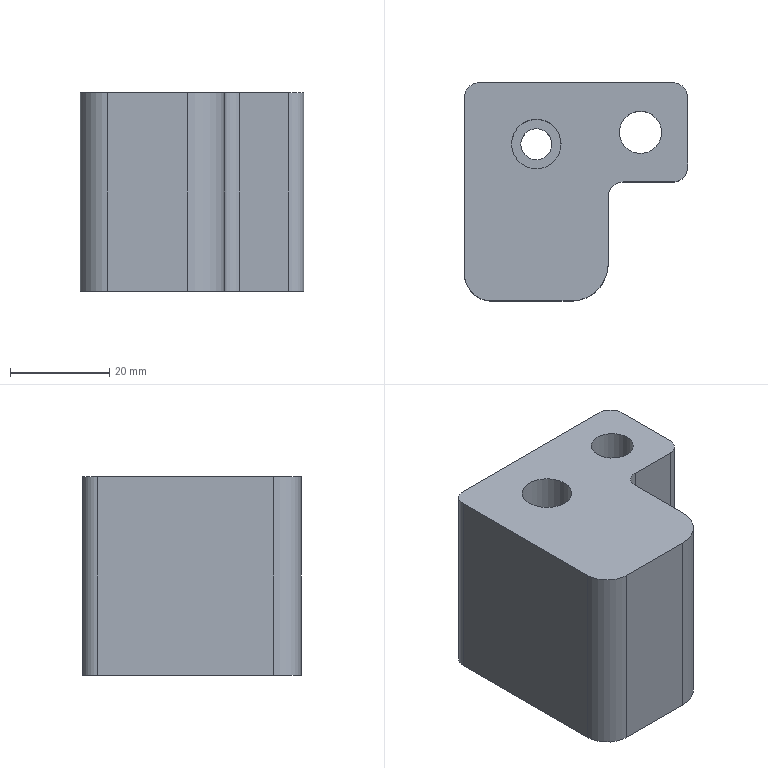Part | NX | features PS-5 2 | 1 solid | 23 faces | box 45 x 44 x 40 mm | volume 54944 mm3 | plane 13 | cylinder 10 | commonest cylinder face diameters 6 x4 6.25 x1 8.5 x1 10 x1 11 x1 14.5 x1
STEP:
#1=CARTESIAN_POINT('',(2416.199,-821.497,860.716));
#2=VERTEX_POINT('',#1);
#3=CARTESIAN_POINT('',(2408.699,-828.997,860.716));
#4=VERTEX_POINT('',#3);
#5=CARTESIAN_POINT('',(2408.699,-821.497,860.716));
#6=DIRECTION('',(0.,0.,1.));
#7=DIRECTION('',(1.,0.,0.));
#8=AXIS2_PLACEMENT_3D('',#5,#6,#7);
#9=CIRCLE('',#8,7.5);
#10=EDGE_CURVE('',#2,#4,#9,.F.);
#11=ORIENTED_EDGE('',*,*,#10,.F.);
#12=CARTESIAN_POINT('',(2416.199,-821.497,900.716));
#13=VERTEX_POINT('',#12);
#14=CARTESIAN_POINT('',(2416.199,-821.497,830.716));
#15=DIRECTION('',(0.,0.,1.));
#16=VECTOR('',#15,1000.);
#17=LINE('',#14,#16);
#18=EDGE_CURVE('',#13,#2,#17,.F.);
#19=ORIENTED_EDGE('',*,*,#18,.F.);
#20=CARTESIAN_POINT('',(2408.699,-828.997,900.716));
#21=VERTEX_POINT('',#20);
#22=CARTESIAN_POINT('',(2408.699,-821.497,900.716));
#23=DIRECTION('',(0.,0.,1.));
#24=DIRECTION('',(1.,0.,0.));
#25=AXIS2_PLACEMENT_3D('',#22,#23,#24);
#26=CIRCLE('',#25,7.5);
#27=EDGE_CURVE('',#13,#21,#26,.F.);
#28=ORIENTED_EDGE('',*,*,#27,.T.);
#29=CARTESIAN_POINT('',(2408.699,-828.997,830.716));
#30=DIRECTION('',(0.,0.,1.));
#31=VECTOR('',#30,1000.);
#32=LINE('',#29,#31);
#33=EDGE_CURVE('',#21,#4,#32,.F.);
#34=ORIENTED_EDGE('',*,*,#33,.T.);
#35=EDGE_LOOP('',(#11,#19,#28,#34));
#36=FACE_BOUND('',#35,.T.);
#37=CARTESIAN_POINT('',(2408.699,-821.497,830.716));
#38=DIRECTION('',(0.,0.,1.));
#39=DIRECTION('',(1.,0.,0.));
#40=AXIS2_PLACEMENT_3D('',#37,#38,#39);
#41=CYLINDRICAL_SURFACE('',#40,7.5);
#42=ADVANCED_FACE('',(#36),#41,.T.);
#43=CARTESIAN_POINT('',(2392.699,-828.997,860.716));
#44=VERTEX_POINT('',#43);
#45=CARTESIAN_POINT('',(2408.699,-828.997,860.716));
#46=DIRECTION('',(1.,0.,0.));
#47=VECTOR('',#46,1000.);
#48=LINE('',#45,#47);
#49=EDGE_CURVE('',#44,#4,#48,.T.);
#50=ORIENTED_EDGE('',*,*,#49,.T.);
#51=ORIENTED_EDGE('',*,*,#33,.F.);
#52=CARTESIAN_POINT('',(2392.699,-828.997,900.716));
#53=VERTEX_POINT('',#52);
#54=CARTESIAN_POINT('',(0.,-828.997,900.716));
#55=DIRECTION('',(-1.,0.,0.));
#56=VECTOR('',#55,1000.);
#57=LINE('',#54,#56);
#58=EDGE_CURVE('',#21,#53,#57,.T.);
#59=ORIENTED_EDGE('',*,*,#58,.T.);
#60=CARTESIAN_POINT('',(2392.699,-828.997,830.716));
#61=DIRECTION('',(0.,0.,1.));
#62=VECTOR('',#61,1000.);
#63=LINE('',#60,#62);
#64=EDGE_CURVE('',#53,#44,#63,.F.);
#65=ORIENTED_EDGE('',*,*,#64,.T.);
#66=EDGE_LOOP('',(#50,#51,#59,#65));
#67=FACE_BOUND('',#66,.T.);
#68=CARTESIAN_POINT('',(2408.699,-828.997,830.716));
#69=DIRECTION('',(0.,1.,0.));
#70=DIRECTION('',(0.,0.,1.));
#71=AXIS2_PLACEMENT_3D('',#68,#69,#70);
#72=PLANE('',#71);
#73=ADVANCED_FACE('',(#67),#72,.F.);
#74=CARTESIAN_POINT('',(2387.199,-823.497,860.716));
#75=VERTEX_POINT('',#74);
#76=CARTESIAN_POINT('',(2392.699,-823.497,860.716));
#77=DIRECTION('',(0.,0.,1.));
#78=DIRECTION('',(1.,0.,0.));
#79=AXIS2_PLACEMENT_3D('',#76,#77,#78);
#80=CIRCLE('',#79,5.5);
#81=EDGE_CURVE('',#75,#44,#80,.T.);
#82=ORIENTED_EDGE('',*,*,#81,.T.);
#83=ORIENTED_EDGE('',*,*,#64,.F.);
#84=CARTESIAN_POINT('',(2387.199,-823.497,900.716));
#85=VERTEX_POINT('',#84);
#86=CARTESIAN_POINT('',(2392.699,-823.497,900.716));
#87=DIRECTION('',(0.,0.,1.));
#88=DIRECTION('',(1.,0.,0.));
#89=AXIS2_PLACEMENT_3D('',#86,#87,#88);
#90=CIRCLE('',#89,5.5);
#91=EDGE_CURVE('',#53,#85,#90,.F.);
#92=ORIENTED_EDGE('',*,*,#91,.T.);
#93=CARTESIAN_POINT('',(2387.199,-823.497,830.716));
#94=DIRECTION('',(0.,0.,1.));
#95=VECTOR('',#94,1000.);
#96=LINE('',#93,#95);
#97=EDGE_CURVE('',#85,#75,#96,.F.);
#98=ORIENTED_EDGE('',*,*,#97,.T.);
#99=EDGE_LOOP('',(#82,#83,#92,#98));
#100=FACE_BOUND('',#99,.T.);
#101=CARTESIAN_POINT('',(2392.699,-823.497,830.716));
#102=DIRECTION('',(0.,0.,1.));
#103=DIRECTION('',(1.,0.,0.));
#104=AXIS2_PLACEMENT_3D('',#101,#102,#103);
#105=CYLINDRICAL_SURFACE('',#104,5.5);
#106=ADVANCED_FACE('',(#100),#105,.T.);
#107=CARTESIAN_POINT('',(2426.949,-794.997,900.716));
#108=VERTEX_POINT('',#107);
#109=CARTESIAN_POINT('',(2422.699,-794.997,900.716));
#110=DIRECTION('',(0.,0.,1.));
#111=DIRECTION('',(1.,0.,0.));
#112=AXIS2_PLACEMENT_3D('',#109,#110,#111);
#113=CIRCLE('',#112,4.25);
#114=EDGE_CURVE('',#108,#108,#113,.T.);
#115=ORIENTED_EDGE('',*,*,#114,.F.);
#116=EDGE_LOOP('',(#115));
#117=FACE_BOUND('',#116,.T.);
#118=CARTESIAN_POINT('',(2432.199,-801.997,900.716));
#119=VERTEX_POINT('',#118);
#120=CARTESIAN_POINT('',(2432.199,-787.997,900.716));
#121=VERTEX_POINT('',#120);
#122=CARTESIAN_POINT('',(2432.199,-790.497,900.716));
#123=DIRECTION('',(0.,1.,0.));
#124=VECTOR('',#123,1000.);
#125=LINE('',#122,#124);
#126=EDGE_CURVE('',#119,#121,#125,.T.);
#127=ORIENTED_EDGE('',*,*,#126,.T.);
#128=CARTESIAN_POINT('',(2429.199,-784.997,900.716));
#129=VERTEX_POINT('',#128);
#130=CARTESIAN_POINT('',(2429.199,-787.997,900.716));
#131=DIRECTION('',(0.,0.,1.));
#132=DIRECTION('',(1.,0.,0.));
#133=AXIS2_PLACEMENT_3D('',#130,#131,#132);
#134=CIRCLE('',#133,3.);
#135=EDGE_CURVE('',#121,#129,#134,.T.);
#136=ORIENTED_EDGE('',*,*,#135,.T.);
#137=CARTESIAN_POINT('',(2390.199,-784.997,900.716));
#138=VERTEX_POINT('',#137);
#139=CARTESIAN_POINT('',(2401.699,-784.997,900.716));
#140=DIRECTION('',(1.,0.,0.));
#141=VECTOR('',#140,1000.);
#142=LINE('',#139,#141);
#143=EDGE_CURVE('',#138,#129,#142,.T.);
#144=ORIENTED_EDGE('',*,*,#143,.F.);
#145=CARTESIAN_POINT('',(2387.199,-787.997,900.716));
#146=VERTEX_POINT('',#145);
#147=CARTESIAN_POINT('',(2390.199,-787.997,900.716));
#148=DIRECTION('',(0.,0.,1.));
#149=DIRECTION('',(1.,0.,0.));
#150=AXIS2_PLACEMENT_3D('',#147,#148,#149);
#151=CIRCLE('',#150,3.);
#152=EDGE_CURVE('',#138,#146,#151,.T.);
#153=ORIENTED_EDGE('',*,*,#152,.T.);
#154=CARTESIAN_POINT('',(2387.199,-823.497,900.716));
#155=DIRECTION('',(0.,-1.,0.));
#156=VECTOR('',#155,1000.);
#157=LINE('',#154,#156);
#158=EDGE_CURVE('',#146,#85,#157,.T.);
#159=ORIENTED_EDGE('',*,*,#158,.T.);
#160=ORIENTED_EDGE('',*,*,#91,.F.);
#161=ORIENTED_EDGE('',*,*,#58,.F.);
#162=ORIENTED_EDGE('',*,*,#27,.F.);
#163=CARTESIAN_POINT('',(2416.199,-807.997,900.716));
#164=VERTEX_POINT('',#163);
#165=CARTESIAN_POINT('',(2416.199,-790.497,900.716));
#166=DIRECTION('',(0.,1.,0.));
#167=VECTOR('',#166,1000.);
#168=LINE('',#165,#167);
#169=EDGE_CURVE('',#13,#164,#168,.T.);
#170=ORIENTED_EDGE('',*,*,#169,.T.);
#171=CARTESIAN_POINT('',(2419.199,-804.997,900.716));
#172=VERTEX_POINT('',#171);
#173=CARTESIAN_POINT('',(2419.199,-807.997,900.716));
#174=DIRECTION('',(0.,0.,1.));
#175=DIRECTION('',(1.,0.,0.));
#176=AXIS2_PLACEMENT_3D('',#173,#174,#175);
#177=CIRCLE('',#176,3.);
#178=EDGE_CURVE('',#164,#172,#177,.F.);
#179=ORIENTED_EDGE('',*,*,#178,.T.);
#180=CARTESIAN_POINT('',(2429.199,-804.997,900.716));
#181=VERTEX_POINT('',#180);
#182=CARTESIAN_POINT('',(2401.699,-804.997,900.716));
#183=DIRECTION('',(1.,0.,0.));
#184=VECTOR('',#183,1000.);
#185=LINE('',#182,#184);
#186=EDGE_CURVE('',#172,#181,#185,.T.);
#187=ORIENTED_EDGE('',*,*,#186,.T.);
#188=CARTESIAN_POINT('',(2429.199,-801.997,900.716));
#189=DIRECTION('',(0.,0.,1.));
#190=DIRECTION('',(1.,0.,0.));
#191=AXIS2_PLACEMENT_3D('',#188,#189,#190);
#192=CIRCLE('',#191,3.);
#193=EDGE_CURVE('',#181,#119,#192,.T.);
#194=ORIENTED_EDGE('',*,*,#193,.T.);
#195=EDGE_LOOP('',(#127,#136,#144,#153,#159,#160,#161,#162,#170,#179,#187,#194));
#196=FACE_BOUND('',#195,.T.);
#197=CARTESIAN_POINT('',(2406.699,-797.347,900.716));
#198=VERTEX_POINT('',#197);
#199=CARTESIAN_POINT('',(2401.699,-797.347,900.716));
#200=DIRECTION('',(0.,0.,1.));
#201=DIRECTION('',(1.,0.,0.));
#202=AXIS2_PLACEMENT_3D('',#199,#200,#201);
#203=CIRCLE('',#202,5.);
#204=EDGE_CURVE('',#198,#198,#203,.T.);
#205=ORIENTED_EDGE('',*,*,#204,.F.);
#206=EDGE_LOOP('',(#205));
#207=FACE_BOUND('',#206,.T.);
#208=CARTESIAN_POINT('',(0.,0.,900.716));
#209=DIRECTION('',(0.,0.,1.));
#210=DIRECTION('',(1.,0.,0.));
#211=AXIS2_PLACEMENT_3D('',#208,#209,#210);
#212=PLANE('',#211);
#213=ADVANCED_FACE('',(#117,#196,#207),#212,.T.);
#214=CARTESIAN_POINT('',(2418.094,-784.997,860.716));
#215=VERTEX_POINT('',#214);
#216=CARTESIAN_POINT('',(2418.094,-789.398,860.716));
#217=VERTEX_POINT('',#216);
#218=CARTESIAN_POINT('',(2418.094,0.,860.716));
#219=DIRECTION('',(0.,-1.,0.));
#220=VECTOR('',#219,1000.);
#221=LINE('',#218,#220);
#222=EDGE_CURVE('',#215,#217,#221,.T.);
#223=ORIENTED_EDGE('',*,*,#222,.T.);
#224=CARTESIAN_POINT('',(2428.978,-798.622,860.716));
#225=VERTEX_POINT('',#224);
#226=CARTESIAN_POINT('',(2422.699,-794.997,860.716));
#227=DIRECTION('',(0.,0.,1.));
#228=DIRECTION('',(1.,0.,0.));
#229=AXIS2_PLACEMENT_3D('',#226,#227,#228);
#230=CIRCLE('',#229,7.25);
#231=EDGE_CURVE('',#217,#225,#230,.T.);
#232=ORIENTED_EDGE('',*,*,#231,.T.);
#233=CARTESIAN_POINT('',(2432.199,-798.622,860.716));
#234=VERTEX_POINT('',#233);
#235=CARTESIAN_POINT('',(0.,-798.622,860.716));
#236=DIRECTION('',(1.,0.,0.));
#237=VECTOR('',#236,1000.);
#238=LINE('',#235,#237);
#239=EDGE_CURVE('',#225,#234,#238,.T.);
#240=ORIENTED_EDGE('',*,*,#239,.T.);
#241=CARTESIAN_POINT('',(2432.199,-801.997,860.716));
#242=VERTEX_POINT('',#241);
#243=CARTESIAN_POINT('',(2432.199,-790.497,860.716));
#244=DIRECTION('',(0.,1.,0.));
#245=VECTOR('',#244,1000.);
#246=LINE('',#243,#245);
#247=EDGE_CURVE('',#242,#234,#246,.T.);
#248=ORIENTED_EDGE('',*,*,#247,.F.);
#249=CARTESIAN_POINT('',(2429.199,-804.997,860.716));
#250=VERTEX_POINT('',#249);
#251=CARTESIAN_POINT('',(2429.199,-801.997,860.716));
#252=DIRECTION('',(0.,0.,1.));
#253=DIRECTION('',(1.,0.,0.));
#254=AXIS2_PLACEMENT_3D('',#251,#252,#253);
#255=CIRCLE('',#254,3.);
#256=EDGE_CURVE('',#242,#250,#255,.F.);
#257=ORIENTED_EDGE('',*,*,#256,.T.);
#258=CARTESIAN_POINT('',(2419.199,-804.997,860.716));
#259=VERTEX_POINT('',#258);
#260=CARTESIAN_POINT('',(0.,-804.997,860.716));
#261=DIRECTION('',(-1.,0.,0.));
#262=VECTOR('',#261,1000.);
#263=LINE('',#260,#262);
#264=EDGE_CURVE('',#259,#250,#263,.F.);
#265=ORIENTED_EDGE('',*,*,#264,.F.);
#266=CARTESIAN_POINT('',(2416.199,-807.997,860.716));
#267=VERTEX_POINT('',#266);
#268=CARTESIAN_POINT('',(2419.199,-807.997,860.716));
#269=DIRECTION('',(0.,0.,1.));
#270=DIRECTION('',(1.,0.,0.));
#271=AXIS2_PLACEMENT_3D('',#268,#269,#270);
#272=CIRCLE('',#271,3.);
#273=EDGE_CURVE('',#259,#267,#272,.T.);
#274=ORIENTED_EDGE('',*,*,#273,.T.);
#275=CARTESIAN_POINT('',(2416.199,-790.497,860.716));
#276=DIRECTION('',(0.,1.,0.));
#277=VECTOR('',#276,1000.);
#278=LINE('',#275,#277);
#279=EDGE_CURVE('',#2,#267,#278,.T.);
#280=ORIENTED_EDGE('',*,*,#279,.F.);
#281=ORIENTED_EDGE('',*,*,#10,.T.);
#282=ORIENTED_EDGE('',*,*,#49,.F.);
#283=ORIENTED_EDGE('',*,*,#81,.F.);
#284=CARTESIAN_POINT('',(2387.199,-787.997,860.716));
#285=VERTEX_POINT('',#284);
#286=CARTESIAN_POINT('',(2387.199,-823.497,860.716));
#287=DIRECTION('',(0.,-1.,0.));
#288=VECTOR('',#287,1000.);
#289=LINE('',#286,#288);
#290=EDGE_CURVE('',#285,#75,#289,.T.);
#291=ORIENTED_EDGE('',*,*,#290,.F.);
#292=CARTESIAN_POINT('',(2390.199,-784.997,860.716));
#293=VERTEX_POINT('',#292);
#294=CARTESIAN_POINT('',(2390.199,-787.997,860.716));
#295=DIRECTION('',(0.,0.,1.));
#296=DIRECTION('',(1.,0.,0.));
#297=AXIS2_PLACEMENT_3D('',#294,#295,#296);
#298=CIRCLE('',#297,3.);
#299=EDGE_CURVE('',#285,#293,#298,.F.);
#300=ORIENTED_EDGE('',*,*,#299,.T.);
#301=CARTESIAN_POINT('',(0.,-784.997,860.716));
#302=DIRECTION('',(-1.,0.,0.));
#303=VECTOR('',#302,1000.);
#304=LINE('',#301,#303);
#305=EDGE_CURVE('',#293,#215,#304,.F.);
#306=ORIENTED_EDGE('',*,*,#305,.T.);
#307=EDGE_LOOP('',(#223,#232,#240,#248,#257,#265,#274,#280,#281,#282,#283,#291,#300,#306));
#308=FACE_BOUND('',#307,.T.);
#309=CARTESIAN_POINT('',(2404.824,-797.347,860.716));
#310=VERTEX_POINT('',#309);
#311=CARTESIAN_POINT('',(2401.699,-797.347,860.716));
#312=DIRECTION('',(0.,0.,1.));
#313=DIRECTION('',(1.,0.,0.));
#314=AXIS2_PLACEMENT_3D('',#311,#312,#313);
#315=CIRCLE('',#314,3.125);
#316=EDGE_CURVE('',#310,#310,#315,.T.);
#317=ORIENTED_EDGE('',*,*,#316,.T.);
#318=EDGE_LOOP('',(#317));
#319=FACE_BOUND('',#318,.T.);
#320=CARTESIAN_POINT('',(0.,0.,860.716));
#321=DIRECTION('',(0.,0.,1.));
#322=DIRECTION('',(1.,0.,0.));
#323=AXIS2_PLACEMENT_3D('',#320,#321,#322);
#324=PLANE('',#323);
#325=ADVANCED_FACE('',(#308,#319),#324,.F.);
#326=ORIENTED_EDGE('',*,*,#158,.F.);
#327=CARTESIAN_POINT('',(2387.199,-787.997,860.716));
#328=DIRECTION('',(0.,0.,1.));
#329=VECTOR('',#328,1000.);
#330=LINE('',#327,#329);
#331=EDGE_CURVE('',#146,#285,#330,.F.);
#332=ORIENTED_EDGE('',*,*,#331,.T.);
#333=ORIENTED_EDGE('',*,*,#290,.T.);
#334=ORIENTED_EDGE('',*,*,#97,.F.);
#335=EDGE_LOOP('',(#326,#332,#333,#334));
#336=FACE_BOUND('',#335,.T.);
#337=CARTESIAN_POINT('',(2387.199,-823.497,830.716));
#338=DIRECTION('',(1.,0.,0.));
#339=DIRECTION('',(0.,0.,-1.));
#340=AXIS2_PLACEMENT_3D('',#337,#338,#339);
#341=PLANE('',#340);
#342=ADVANCED_FACE('',(#336),#341,.F.);
#343=ORIENTED_EDGE('',*,*,#279,.T.);
#344=CARTESIAN_POINT('',(2416.199,-807.997,890.716));
#345=DIRECTION('',(0.,0.,-1.));
#346=VECTOR('',#345,1000.);
#347=LINE('',#344,#346);
#348=EDGE_CURVE('',#267,#164,#347,.F.);
#349=ORIENTED_EDGE('',*,*,#348,.T.);
#350=ORIENTED_EDGE('',*,*,#169,.F.);
#351=ORIENTED_EDGE('',*,*,#18,.T.);
#352=EDGE_LOOP('',(#343,#349,#350,#351));
#353=FACE_BOUND('',#352,.T.);
#354=CARTESIAN_POINT('',(2416.199,-790.497,830.716));
#355=DIRECTION('',(-1.,0.,0.));
#356=DIRECTION('',(0.,0.,1.));
#357=AXIS2_PLACEMENT_3D('',#354,#355,#356);
#358=PLANE('',#357);
#359=ADVANCED_FACE('',(#353),#358,.F.);
#360=ORIENTED_EDGE('',*,*,#264,.T.);
#361=CARTESIAN_POINT('',(2429.199,-804.997,875.716));
#362=DIRECTION('',(0.,0.,1.));
#363=VECTOR('',#362,1000.);
#364=LINE('',#361,#363);
#365=EDGE_CURVE('',#250,#181,#364,.T.);
#366=ORIENTED_EDGE('',*,*,#365,.T.);
#367=ORIENTED_EDGE('',*,*,#186,.F.);
#368=CARTESIAN_POINT('',(2419.199,-804.997,860.716));
#369=DIRECTION('',(0.,0.,-1.));
#370=VECTOR('',#369,1000.);
#371=LINE('',#368,#370);
#372=EDGE_CURVE('',#172,#259,#371,.T.);
#373=ORIENTED_EDGE('',*,*,#372,.T.);
#374=EDGE_LOOP('',(#360,#366,#367,#373));
#375=FACE_BOUND('',#374,.T.);
#376=CARTESIAN_POINT('',(2401.699,-804.997,875.716));
#377=DIRECTION('',(0.,1.,0.));
#378=DIRECTION('',(0.,0.,1.));
#379=AXIS2_PLACEMENT_3D('',#376,#377,#378);
#380=PLANE('',#379);
#381=ADVANCED_FACE('',(#375),#380,.F.);
#382=CARTESIAN_POINT('',(2398.574,-797.347,871.716));
#383=VERTEX_POINT('',#382);
#384=CARTESIAN_POINT('',(2401.699,-797.347,871.716));
#385=DIRECTION('',(0.,0.,-1.));
#386=DIRECTION('',(-1.,0.,0.));
#387=AXIS2_PLACEMENT_3D('',#384,#385,#386);
#388=CIRCLE('',#387,3.125);
#389=EDGE_CURVE('',#383,#383,#388,.T.);
#390=ORIENTED_EDGE('',*,*,#389,.T.);
#391=EDGE_LOOP('',(#390));
#392=FACE_BOUND('',#391,.T.);
#393=CARTESIAN_POINT('',(2406.699,-797.347,871.716));
#394=VERTEX_POINT('',#393);
#395=CARTESIAN_POINT('',(2401.699,-797.347,871.716));
#396=DIRECTION('',(0.,0.,1.));
#397=DIRECTION('',(1.,0.,0.));
#398=AXIS2_PLACEMENT_3D('',#395,#396,#397);
#399=CIRCLE('',#398,5.);
#400=EDGE_CURVE('',#394,#394,#399,.F.);
#401=ORIENTED_EDGE('',*,*,#400,.F.);
#402=EDGE_LOOP('',(#401));
#403=FACE_BOUND('',#402,.T.);
#404=CARTESIAN_POINT('',(2401.699,-797.347,871.716));
#405=DIRECTION('',(0.,0.,-1.));
#406=DIRECTION('',(-1.,0.,0.));
#407=AXIS2_PLACEMENT_3D('',#404,#405,#406);
#408=PLANE('',#407);
#409=ADVANCED_FACE('',(#392,#403),#408,.F.);
#410=ORIENTED_EDGE('',*,*,#389,.F.);
#411=EDGE_LOOP('',(#410));
#412=FACE_BOUND('',#411,.T.);
#413=ORIENTED_EDGE('',*,*,#316,.F.);
#414=EDGE_LOOP('',(#413));
#415=FACE_BOUND('',#414,.T.);
#416=CARTESIAN_POINT('',(2401.699,-797.347,935.716));
#417=DIRECTION('',(0.,0.,-1.));
#418=DIRECTION('',(1.,0.,0.));
#419=AXIS2_PLACEMENT_3D('',#416,#417,#418);
#420=CYLINDRICAL_SURFACE('',#419,3.125);
#421=ADVANCED_FACE('',(#412,#415),#420,.F.);
#422=ORIENTED_EDGE('',*,*,#247,.T.);
#423=CARTESIAN_POINT('',(2432.199,-798.622,871.716));
#424=VERTEX_POINT('',#423);
#425=CARTESIAN_POINT('',(2432.199,-798.622,830.716));
#426=DIRECTION('',(0.,0.,1.));
#427=VECTOR('',#426,1000.);
#428=LINE('',#425,#427);
#429=EDGE_CURVE('',#234,#424,#428,.T.);
#430=ORIENTED_EDGE('',*,*,#429,.T.);
#431=CARTESIAN_POINT('',(2432.199,-787.997,871.716));
#432=VERTEX_POINT('',#431);
#433=CARTESIAN_POINT('',(2432.199,-790.497,871.716));
#434=DIRECTION('',(0.,1.,0.));
#435=VECTOR('',#434,1000.);
#436=LINE('',#433,#435);
#437=EDGE_CURVE('',#424,#432,#436,.T.);
#438=ORIENTED_EDGE('',*,*,#437,.T.);
#439=CARTESIAN_POINT('',(2432.199,-787.997,890.716));
#440=DIRECTION('',(0.,0.,-1.));
#441=VECTOR('',#440,1000.);
#442=LINE('',#439,#441);
#443=EDGE_CURVE('',#432,#121,#442,.F.);
#444=ORIENTED_EDGE('',*,*,#443,.T.);
#445=ORIENTED_EDGE('',*,*,#126,.F.);
#446=CARTESIAN_POINT('',(2432.199,-801.997,830.716));
#447=DIRECTION('',(0.,0.,1.));
#448=VECTOR('',#447,1000.);
#449=LINE('',#446,#448);
#450=EDGE_CURVE('',#119,#242,#449,.F.);
#451=ORIENTED_EDGE('',*,*,#450,.T.);
#452=EDGE_LOOP('',(#422,#430,#438,#444,#445,#451));
#453=FACE_BOUND('',#452,.T.);
#454=CARTESIAN_POINT('',(2432.199,-790.497,830.716));
#455=DIRECTION('',(-1.,0.,0.));
#456=DIRECTION('',(0.,0.,1.));
#457=AXIS2_PLACEMENT_3D('',#454,#455,#456);
#458=PLANE('',#457);
#459=ADVANCED_FACE('',(#453),#458,.F.);
#460=ORIENTED_EDGE('',*,*,#204,.T.);
#461=EDGE_LOOP('',(#460));
#462=FACE_BOUND('',#461,.T.);
#463=ORIENTED_EDGE('',*,*,#400,.T.);
#464=EDGE_LOOP('',(#463));
#465=FACE_BOUND('',#464,.T.);
#466=CARTESIAN_POINT('',(2401.699,-797.347,935.716));
#467=DIRECTION('',(0.,0.,-1.));
#468=DIRECTION('',(1.,0.,0.));
#469=AXIS2_PLACEMENT_3D('',#466,#467,#468);
#470=CYLINDRICAL_SURFACE('',#469,5.);
#471=ADVANCED_FACE('',(#462,#465),#470,.F.);
#472=CARTESIAN_POINT('',(2418.094,-784.997,871.716));
#473=VERTEX_POINT('',#472);
#474=CARTESIAN_POINT('',(2418.094,-784.997,875.716));
#475=DIRECTION('',(0.,0.,1.));
#476=VECTOR('',#475,1000.);
#477=LINE('',#474,#476);
#478=EDGE_CURVE('',#215,#473,#477,.T.);
#479=ORIENTED_EDGE('',*,*,#478,.F.);
#480=ORIENTED_EDGE('',*,*,#305,.F.);
#481=CARTESIAN_POINT('',(2390.199,-784.997,890.716));
#482=DIRECTION('',(0.,0.,1.));
#483=VECTOR('',#482,1000.);
#484=LINE('',#481,#483);
#485=EDGE_CURVE('',#293,#138,#484,.T.);
#486=ORIENTED_EDGE('',*,*,#485,.T.);
#487=ORIENTED_EDGE('',*,*,#143,.T.);
#488=CARTESIAN_POINT('',(2429.199,-784.997,871.716));
#489=VERTEX_POINT('',#488);
#490=CARTESIAN_POINT('',(2429.199,-784.997,860.716));
#491=DIRECTION('',(0.,0.,-1.));
#492=VECTOR('',#491,1000.);
#493=LINE('',#490,#492);
#494=EDGE_CURVE('',#129,#489,#493,.T.);
#495=ORIENTED_EDGE('',*,*,#494,.T.);
#496=CARTESIAN_POINT('',(2401.699,-784.997,871.716));
#497=DIRECTION('',(1.,0.,0.));
#498=VECTOR('',#497,1000.);
#499=LINE('',#496,#498);
#500=EDGE_CURVE('',#473,#489,#499,.T.);
#501=ORIENTED_EDGE('',*,*,#500,.F.);
#502=EDGE_LOOP('',(#479,#480,#486,#487,#495,#501));
#503=FACE_BOUND('',#502,.T.);
#504=CARTESIAN_POINT('',(2401.699,-784.997,875.716));
#505=DIRECTION('',(0.,1.,0.));
#506=DIRECTION('',(0.,0.,1.));
#507=AXIS2_PLACEMENT_3D('',#504,#505,#506);
#508=PLANE('',#507);
#509=ADVANCED_FACE('',(#503),#508,.T.);
#510=ORIENTED_EDGE('',*,*,#256,.F.);
#511=ORIENTED_EDGE('',*,*,#450,.F.);
#512=ORIENTED_EDGE('',*,*,#193,.F.);
#513=ORIENTED_EDGE('',*,*,#365,.F.);
#514=EDGE_LOOP('',(#510,#511,#512,#513));
#515=FACE_BOUND('',#514,.T.);
#516=CARTESIAN_POINT('',(2429.199,-801.997,875.716));
#517=DIRECTION('',(0.,0.,1.));
#518=DIRECTION('',(1.,0.,0.));
#519=AXIS2_PLACEMENT_3D('',#516,#517,#518);
#520=CYLINDRICAL_SURFACE('',#519,3.);
#521=ADVANCED_FACE('',(#515),#520,.T.);
#522=ORIENTED_EDGE('',*,*,#178,.F.);
#523=ORIENTED_EDGE('',*,*,#348,.F.);
#524=ORIENTED_EDGE('',*,*,#273,.F.);
#525=ORIENTED_EDGE('',*,*,#372,.F.);
#526=EDGE_LOOP('',(#522,#523,#524,#525));
#527=FACE_BOUND('',#526,.T.);
#528=CARTESIAN_POINT('',(2419.199,-807.997,875.716));
#529=DIRECTION('',(0.,0.,1.));
#530=DIRECTION('',(1.,0.,0.));
#531=AXIS2_PLACEMENT_3D('',#528,#529,#530);
#532=CYLINDRICAL_SURFACE('',#531,3.);
#533=ADVANCED_FACE('',(#527),#532,.F.);
#534=CARTESIAN_POINT('',(2429.199,-787.997,871.716));
#535=DIRECTION('',(0.,0.,1.));
#536=DIRECTION('',(1.,0.,0.));
#537=AXIS2_PLACEMENT_3D('',#534,#535,#536);
#538=CIRCLE('',#537,3.);
#539=EDGE_CURVE('',#489,#432,#538,.F.);
#540=ORIENTED_EDGE('',*,*,#539,.F.);
#541=ORIENTED_EDGE('',*,*,#494,.F.);
#542=ORIENTED_EDGE('',*,*,#135,.F.);
#543=ORIENTED_EDGE('',*,*,#443,.F.);
#544=EDGE_LOOP('',(#540,#541,#542,#543));
#545=FACE_BOUND('',#544,.T.);
#546=CARTESIAN_POINT('',(2429.199,-787.997,875.716));
#547=DIRECTION('',(0.,0.,1.));
#548=DIRECTION('',(1.,0.,0.));
#549=AXIS2_PLACEMENT_3D('',#546,#547,#548);
#550=CYLINDRICAL_SURFACE('',#549,3.);
#551=ADVANCED_FACE('',(#545),#550,.T.);
#552=ORIENTED_EDGE('',*,*,#299,.F.);
#553=ORIENTED_EDGE('',*,*,#331,.F.);
#554=ORIENTED_EDGE('',*,*,#152,.F.);
#555=ORIENTED_EDGE('',*,*,#485,.F.);
#556=EDGE_LOOP('',(#552,#553,#554,#555));
#557=FACE_BOUND('',#556,.T.);
#558=CARTESIAN_POINT('',(2390.199,-787.997,875.716));
#559=DIRECTION('',(0.,0.,-1.));
#560=DIRECTION('',(-1.,0.,0.));
#561=AXIS2_PLACEMENT_3D('',#558,#559,#560);
#562=CYLINDRICAL_SURFACE('',#561,3.);
#563=ADVANCED_FACE('',(#557),#562,.T.);
#564=ORIENTED_EDGE('',*,*,#239,.F.);
#565=CARTESIAN_POINT('',(2428.978,-798.622,871.716));
#566=VERTEX_POINT('',#565);
#567=CARTESIAN_POINT('',(2428.978,-798.622,871.716));
#568=DIRECTION('',(0.,0.,-1.));
#569=VECTOR('',#568,1000.);
#570=LINE('',#567,#569);
#571=EDGE_CURVE('',#225,#566,#570,.F.);
#572=ORIENTED_EDGE('',*,*,#571,.T.);
#573=CARTESIAN_POINT('',(2431.094,-798.622,871.716));
#574=DIRECTION('',(1.,0.,0.));
#575=VECTOR('',#574,1000.);
#576=LINE('',#573,#575);
#577=EDGE_CURVE('',#424,#566,#576,.F.);
#578=ORIENTED_EDGE('',*,*,#577,.F.);
#579=ORIENTED_EDGE('',*,*,#429,.F.);
#580=EDGE_LOOP('',(#564,#572,#578,#579));
#581=FACE_BOUND('',#580,.T.);
#582=CARTESIAN_POINT('',(2431.094,-798.622,851.716));
#583=DIRECTION('',(0.,-1.,0.));
#584=DIRECTION('',(0.,0.,-1.));
#585=AXIS2_PLACEMENT_3D('',#582,#583,#584);
#586=PLANE('',#585);
#587=ADVANCED_FACE('',(#581),#586,.F.);
#588=CARTESIAN_POINT('',(2418.094,-789.398,871.716));
#589=VERTEX_POINT('',#588);
#590=CARTESIAN_POINT('',(2418.094,-784.622,871.716));
#591=DIRECTION('',(0.,-1.,0.));
#592=VECTOR('',#591,1000.);
#593=LINE('',#590,#592);
#594=EDGE_CURVE('',#589,#473,#593,.F.);
#595=ORIENTED_EDGE('',*,*,#594,.F.);
#596=CARTESIAN_POINT('',(2418.094,-789.398,871.716));
#597=DIRECTION('',(0.,0.,-1.));
#598=VECTOR('',#597,1000.);
#599=LINE('',#596,#598);
#600=EDGE_CURVE('',#589,#217,#599,.T.);
#601=ORIENTED_EDGE('',*,*,#600,.T.);
#602=ORIENTED_EDGE('',*,*,#222,.F.);
#603=ORIENTED_EDGE('',*,*,#478,.T.);
#604=EDGE_LOOP('',(#595,#601,#602,#603));
#605=FACE_BOUND('',#604,.T.);
#606=CARTESIAN_POINT('',(2418.094,-784.622,851.716));
#607=DIRECTION('',(-1.,0.,0.));
#608=DIRECTION('',(0.,0.,1.));
#609=AXIS2_PLACEMENT_3D('',#606,#607,#608);
#610=PLANE('',#609);
#611=ADVANCED_FACE('',(#605),#610,.F.);
#612=ORIENTED_EDGE('',*,*,#577,.T.);
#613=CARTESIAN_POINT('',(2422.699,-794.997,871.716));
#614=DIRECTION('',(0.,0.,1.));
#615=DIRECTION('',(1.,0.,0.));
#616=AXIS2_PLACEMENT_3D('',#613,#614,#615);
#617=CIRCLE('',#616,7.25);
#618=EDGE_CURVE('',#566,#589,#617,.T.);
#619=ORIENTED_EDGE('',*,*,#618,.T.);
#620=ORIENTED_EDGE('',*,*,#594,.T.);
#621=ORIENTED_EDGE('',*,*,#500,.T.);
#622=ORIENTED_EDGE('',*,*,#539,.T.);
#623=ORIENTED_EDGE('',*,*,#437,.F.);
#624=EDGE_LOOP('',(#612,#619,#620,#621,#622,#623));
#625=FACE_BOUND('',#624,.T.);
#626=CARTESIAN_POINT('',(2431.094,-784.622,871.716));
#627=DIRECTION('',(0.,0.,1.));
#628=DIRECTION('',(1.,0.,0.));
#629=AXIS2_PLACEMENT_3D('',#626,#627,#628);
#630=PLANE('',#629);
#631=ADVANCED_FACE('',(#625),#630,.F.);
#632=CARTESIAN_POINT('',(2415.449,-794.997,881.716));
#633=VERTEX_POINT('',#632);
#634=CARTESIAN_POINT('',(2422.699,-794.997,881.716));
#635=DIRECTION('',(0.,0.,-1.));
#636=DIRECTION('',(-1.,0.,0.));
#637=AXIS2_PLACEMENT_3D('',#634,#635,#636);
#638=CIRCLE('',#637,7.25);
#639=EDGE_CURVE('',#633,#633,#638,.F.);
#640=ORIENTED_EDGE('',*,*,#639,.T.);
#641=EDGE_LOOP('',(#640));
#642=FACE_BOUND('',#641,.T.);
#643=ORIENTED_EDGE('',*,*,#600,.F.);
#644=ORIENTED_EDGE('',*,*,#618,.F.);
#645=ORIENTED_EDGE('',*,*,#571,.F.);
#646=ORIENTED_EDGE('',*,*,#231,.F.);
#647=EDGE_LOOP('',(#643,#644,#645,#646));
#648=FACE_BOUND('',#647,.T.);
#649=CARTESIAN_POINT('',(2422.699,-794.997,871.716));
#650=DIRECTION('',(0.,0.,-1.));
#651=DIRECTION('',(-1.,0.,0.));
#652=AXIS2_PLACEMENT_3D('',#649,#650,#651);
#653=CYLINDRICAL_SURFACE('',#652,7.25);
#654=ADVANCED_FACE('',(#642,#648),#653,.F.);
#655=ORIENTED_EDGE('',*,*,#114,.T.);
#656=EDGE_LOOP('',(#655));
#657=FACE_BOUND('',#656,.T.);
#658=CARTESIAN_POINT('',(2418.449,-794.997,881.716));
#659=VERTEX_POINT('',#658);
#660=CARTESIAN_POINT('',(2422.699,-794.997,881.716));
#661=DIRECTION('',(0.,0.,-1.));
#662=DIRECTION('',(-1.,0.,0.));
#663=AXIS2_PLACEMENT_3D('',#660,#661,#662);
#664=CIRCLE('',#663,4.25);
#665=EDGE_CURVE('',#659,#659,#664,.T.);
#666=ORIENTED_EDGE('',*,*,#665,.T.);
#667=EDGE_LOOP('',(#666));
#668=FACE_BOUND('',#667,.T.);
#669=CARTESIAN_POINT('',(2422.699,-794.997,891.716));
#670=DIRECTION('',(0.,0.,-1.));
#671=DIRECTION('',(-1.,0.,0.));
#672=AXIS2_PLACEMENT_3D('',#669,#670,#671);
#673=CYLINDRICAL_SURFACE('',#672,4.25);
#674=ADVANCED_FACE('',(#657,#668),#673,.F.);
#675=ORIENTED_EDGE('',*,*,#665,.F.);
#676=EDGE_LOOP('',(#675));
#677=FACE_BOUND('',#676,.T.);
#678=ORIENTED_EDGE('',*,*,#639,.F.);
#679=EDGE_LOOP('',(#678));
#680=FACE_BOUND('',#679,.T.);
#681=CARTESIAN_POINT('',(2422.699,-794.997,881.716));
#682=DIRECTION('',(0.,0.,-1.));
#683=DIRECTION('',(-1.,0.,0.));
#684=AXIS2_PLACEMENT_3D('',#681,#682,#683);
#685=PLANE('',#684);
#686=ADVANCED_FACE('',(#677,#680),#685,.T.);
#687=CLOSED_SHELL('',(#42,#73,#106,#213,#325,#342,#359,#381,#409,#421,#459,#471,#509,#521,#533,#551,#563,#587,#611,#631,#654,#674,#686));
#688=MANIFOLD_SOLID_BREP('',#687);
#689=(LENGTH_UNIT()NAMED_UNIT(*)SI_UNIT(.MILLI.,.METRE.));
#690=UNCERTAINTY_MEASURE_WITH_UNIT(LENGTH_MEASURE(0.00001),#689,'','');
#691=(NAMED_UNIT(*)PLANE_ANGLE_UNIT()SI_UNIT($,.RADIAN.));
#692=(NAMED_UNIT(*)SI_UNIT($,.STERADIAN.)SOLID_ANGLE_UNIT());
#693=(GEOMETRIC_REPRESENTATION_CONTEXT(3)GLOBAL_UNCERTAINTY_ASSIGNED_CONTEXT((#690))GLOBAL_UNIT_ASSIGNED_CONTEXT((#689,#691,#692))REPRESENTATION_CONTEXT('',''));
#694=ADVANCED_BREP_SHAPE_REPRESENTATION('',(#688),#693);